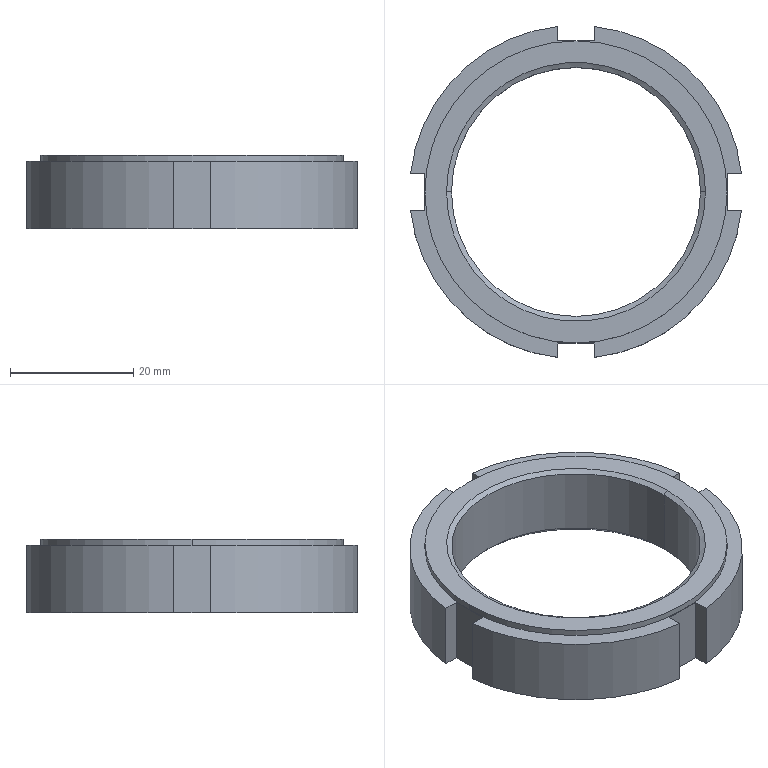Part | STEP file | 201100_M42x1_5_HI | 1 solid | 30 faces | box 53.666 x 53.666 x 12 mm | volume 11002 mm3 | plane 18 | cylinder 8 | cone 4 | commonest cylinder face diameters 54 x4 40.376 x2 49 x2